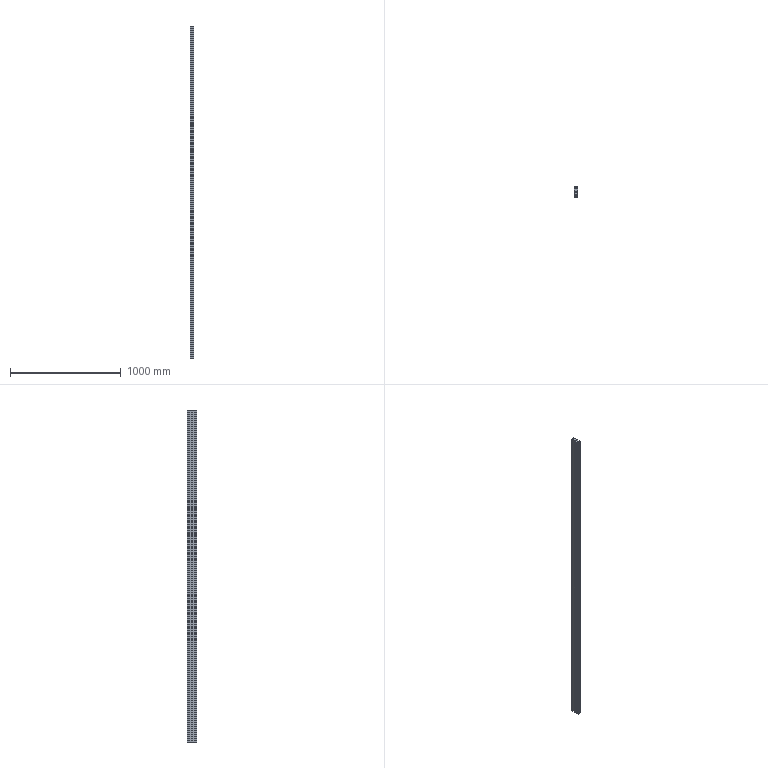Part | SolidWorks | features BaseBody 1 | 1 solid | 38 faces | box 30 x 90 x 3000 mm | volume 6756000 mm3 | plane 38
STEP:
#1=CARTESIAN_POINT('',(8.,-4.,3000.));
#2=VERTEX_POINT('',#1);
#3=CARTESIAN_POINT('',(15.,-4.,3000.));
#4=VERTEX_POINT('',#3);
#5=CARTESIAN_POINT('',(8.,-4.,3000.));
#6=DIRECTION('',(1.,0.,0.));
#7=VECTOR('',#6,1000.);
#8=LINE('',#5,#7);
#9=EDGE_CURVE('',#2,#4,#8,.T.);
#10=ORIENTED_EDGE('',*,*,#9,.T.);
#11=CARTESIAN_POINT('',(15.,-4.,0.));
#12=VERTEX_POINT('',#11);
#13=CARTESIAN_POINT('',(15.,-4.,0.));
#14=DIRECTION('',(0.,0.,1.));
#15=VECTOR('',#14,1000.);
#16=LINE('',#13,#15);
#17=EDGE_CURVE('',#12,#4,#16,.T.);
#18=ORIENTED_EDGE('',*,*,#17,.F.);
#19=CARTESIAN_POINT('',(8.,-4.,0.));
#20=VERTEX_POINT('',#19);
#21=CARTESIAN_POINT('',(8.,-4.,0.));
#22=DIRECTION('',(1.,0.,0.));
#23=VECTOR('',#22,1000.);
#24=LINE('',#21,#23);
#25=EDGE_CURVE('',#20,#12,#24,.T.);
#26=ORIENTED_EDGE('',*,*,#25,.F.);
#27=CARTESIAN_POINT('',(8.,-4.,0.));
#28=DIRECTION('',(0.,0.,1.));
#29=VECTOR('',#28,1000.);
#30=LINE('',#27,#29);
#31=EDGE_CURVE('',#20,#2,#30,.T.);
#32=ORIENTED_EDGE('',*,*,#31,.T.);
#33=EDGE_LOOP('',(#10,#18,#26,#32));
#34=FACE_OUTER_BOUND('',#33,.T.);
#35=CARTESIAN_POINT('',(8.,-4.,0.));
#36=DIRECTION('',(0.,-1.,0.));
#37=DIRECTION('',(0.,0.,-1.));
#38=AXIS2_PLACEMENT_3D('',#35,#36,#37);
#39=PLANE('',#38);
#40=ADVANCED_FACE('',(#34),#39,.F.);
#41=CARTESIAN_POINT('',(15.,4.,3000.));
#42=VERTEX_POINT('',#41);
#43=CARTESIAN_POINT('',(8.,4.,3000.));
#44=VERTEX_POINT('',#43);
#45=CARTESIAN_POINT('',(8.,4.,3000.));
#46=DIRECTION('',(-1.,0.,0.));
#47=VECTOR('',#46,1000.);
#48=LINE('',#45,#47);
#49=EDGE_CURVE('',#42,#44,#48,.T.);
#50=ORIENTED_EDGE('',*,*,#49,.T.);
#51=CARTESIAN_POINT('',(8.,4.,0.));
#52=VERTEX_POINT('',#51);
#53=CARTESIAN_POINT('',(8.,4.,0.));
#54=DIRECTION('',(0.,0.,1.));
#55=VECTOR('',#54,1000.);
#56=LINE('',#53,#55);
#57=EDGE_CURVE('',#52,#44,#56,.T.);
#58=ORIENTED_EDGE('',*,*,#57,.F.);
#59=CARTESIAN_POINT('',(15.,4.,0.));
#60=VERTEX_POINT('',#59);
#61=CARTESIAN_POINT('',(8.,4.,0.));
#62=DIRECTION('',(-1.,0.,0.));
#63=VECTOR('',#62,1000.);
#64=LINE('',#61,#63);
#65=EDGE_CURVE('',#60,#52,#64,.T.);
#66=ORIENTED_EDGE('',*,*,#65,.F.);
#67=CARTESIAN_POINT('',(15.,4.,0.));
#68=DIRECTION('',(0.,0.,1.));
#69=VECTOR('',#68,1000.);
#70=LINE('',#67,#69);
#71=EDGE_CURVE('',#60,#42,#70,.T.);
#72=ORIENTED_EDGE('',*,*,#71,.T.);
#73=EDGE_LOOP('',(#50,#58,#66,#72));
#74=FACE_OUTER_BOUND('',#73,.T.);
#75=CARTESIAN_POINT('',(8.,4.,0.));
#76=DIRECTION('',(0.,1.,0.));
#77=DIRECTION('',(1.,0.,0.));
#78=AXIS2_PLACEMENT_3D('',#75,#76,#77);
#79=PLANE('',#78);
#80=ADVANCED_FACE('',(#74),#79,.F.);
#81=CARTESIAN_POINT('',(8.,-4.,3000.));
#82=DIRECTION('',(0.,-1.,0.));
#83=VECTOR('',#82,1000.);
#84=LINE('',#81,#83);
#85=EDGE_CURVE('',#44,#2,#84,.T.);
#86=ORIENTED_EDGE('',*,*,#85,.T.);
#87=ORIENTED_EDGE('',*,*,#31,.F.);
#88=CARTESIAN_POINT('',(8.,-4.,0.));
#89=DIRECTION('',(0.,-1.,0.));
#90=VECTOR('',#89,1000.);
#91=LINE('',#88,#90);
#92=EDGE_CURVE('',#52,#20,#91,.T.);
#93=ORIENTED_EDGE('',*,*,#92,.F.);
#94=ORIENTED_EDGE('',*,*,#57,.T.);
#95=EDGE_LOOP('',(#86,#87,#93,#94));
#96=FACE_OUTER_BOUND('',#95,.T.);
#97=CARTESIAN_POINT('',(8.,-4.,0.));
#98=DIRECTION('',(-1.,0.,0.));
#99=DIRECTION('',(0.,0.,1.));
#100=AXIS2_PLACEMENT_3D('',#97,#98,#99);
#101=PLANE('',#100);
#102=ADVANCED_FACE('',(#96),#101,.F.);
#103=CARTESIAN_POINT('',(-15.,-4.,3000.));
#104=VERTEX_POINT('',#103);
#105=CARTESIAN_POINT('',(-8.,-4.,3000.));
#106=VERTEX_POINT('',#105);
#107=CARTESIAN_POINT('',(-15.,-4.,3000.));
#108=DIRECTION('',(1.,0.,0.));
#109=VECTOR('',#108,1000.);
#110=LINE('',#107,#109);
#111=EDGE_CURVE('',#104,#106,#110,.T.);
#112=ORIENTED_EDGE('',*,*,#111,.T.);
#113=CARTESIAN_POINT('',(-8.,-4.,0.));
#114=VERTEX_POINT('',#113);
#115=CARTESIAN_POINT('',(-8.,-4.,0.));
#116=DIRECTION('',(0.,0.,1.));
#117=VECTOR('',#116,1000.);
#118=LINE('',#115,#117);
#119=EDGE_CURVE('',#114,#106,#118,.T.);
#120=ORIENTED_EDGE('',*,*,#119,.F.);
#121=CARTESIAN_POINT('',(-15.,-4.,0.));
#122=VERTEX_POINT('',#121);
#123=CARTESIAN_POINT('',(-15.,-4.,0.));
#124=DIRECTION('',(1.,0.,0.));
#125=VECTOR('',#124,1000.);
#126=LINE('',#123,#125);
#127=EDGE_CURVE('',#122,#114,#126,.T.);
#128=ORIENTED_EDGE('',*,*,#127,.F.);
#129=CARTESIAN_POINT('',(-15.,-4.,0.));
#130=DIRECTION('',(0.,0.,1.));
#131=VECTOR('',#130,1000.);
#132=LINE('',#129,#131);
#133=EDGE_CURVE('',#122,#104,#132,.T.);
#134=ORIENTED_EDGE('',*,*,#133,.T.);
#135=EDGE_LOOP('',(#112,#120,#128,#134));
#136=FACE_OUTER_BOUND('',#135,.T.);
#137=CARTESIAN_POINT('',(-15.,-4.,0.));
#138=DIRECTION('',(0.,-1.,0.));
#139=DIRECTION('',(0.,0.,-1.));
#140=AXIS2_PLACEMENT_3D('',#137,#138,#139);
#141=PLANE('',#140);
#142=ADVANCED_FACE('',(#136),#141,.F.);
#143=CARTESIAN_POINT('',(-8.,4.,3000.));
#144=VERTEX_POINT('',#143);
#145=CARTESIAN_POINT('',(-8.,-4.,3000.));
#146=DIRECTION('',(0.,1.,0.));
#147=VECTOR('',#146,1000.);
#148=LINE('',#145,#147);
#149=EDGE_CURVE('',#106,#144,#148,.T.);
#150=ORIENTED_EDGE('',*,*,#149,.T.);
#151=CARTESIAN_POINT('',(-8.,4.,0.));
#152=VERTEX_POINT('',#151);
#153=CARTESIAN_POINT('',(-8.,4.,0.));
#154=DIRECTION('',(0.,0.,1.));
#155=VECTOR('',#154,1000.);
#156=LINE('',#153,#155);
#157=EDGE_CURVE('',#152,#144,#156,.T.);
#158=ORIENTED_EDGE('',*,*,#157,.F.);
#159=CARTESIAN_POINT('',(-8.,-4.,0.));
#160=DIRECTION('',(0.,1.,0.));
#161=VECTOR('',#160,1000.);
#162=LINE('',#159,#161);
#163=EDGE_CURVE('',#114,#152,#162,.T.);
#164=ORIENTED_EDGE('',*,*,#163,.F.);
#165=ORIENTED_EDGE('',*,*,#119,.T.);
#166=EDGE_LOOP('',(#150,#158,#164,#165));
#167=FACE_OUTER_BOUND('',#166,.T.);
#168=CARTESIAN_POINT('',(-8.,-4.,0.));
#169=DIRECTION('',(1.,0.,0.));
#170=DIRECTION('',(0.,1.,0.));
#171=AXIS2_PLACEMENT_3D('',#168,#169,#170);
#172=PLANE('',#171);
#173=ADVANCED_FACE('',(#167),#172,.F.);
#174=CARTESIAN_POINT('',(-15.,4.,3000.));
#175=VERTEX_POINT('',#174);
#176=CARTESIAN_POINT('',(-15.,4.,3000.));
#177=DIRECTION('',(-1.,0.,0.));
#178=VECTOR('',#177,1000.);
#179=LINE('',#176,#178);
#180=EDGE_CURVE('',#144,#175,#179,.T.);
#181=ORIENTED_EDGE('',*,*,#180,.T.);
#182=CARTESIAN_POINT('',(-15.,4.,0.));
#183=VERTEX_POINT('',#182);
#184=CARTESIAN_POINT('',(-15.,4.,0.));
#185=DIRECTION('',(0.,0.,1.));
#186=VECTOR('',#185,1000.);
#187=LINE('',#184,#186);
#188=EDGE_CURVE('',#183,#175,#187,.T.);
#189=ORIENTED_EDGE('',*,*,#188,.F.);
#190=CARTESIAN_POINT('',(-15.,4.,0.));
#191=DIRECTION('',(-1.,0.,0.));
#192=VECTOR('',#191,1000.);
#193=LINE('',#190,#192);
#194=EDGE_CURVE('',#152,#183,#193,.T.);
#195=ORIENTED_EDGE('',*,*,#194,.F.);
#196=ORIENTED_EDGE('',*,*,#157,.T.);
#197=EDGE_LOOP('',(#181,#189,#195,#196));
#198=FACE_OUTER_BOUND('',#197,.T.);
#199=CARTESIAN_POINT('',(-15.,4.,0.));
#200=DIRECTION('',(0.,1.,0.));
#201=DIRECTION('',(1.,0.,0.));
#202=AXIS2_PLACEMENT_3D('',#199,#200,#201);
#203=PLANE('',#202);
#204=ADVANCED_FACE('',(#198),#203,.F.);
#205=CARTESIAN_POINT('',(15.,-26.,3000.));
#206=VERTEX_POINT('',#205);
#207=CARTESIAN_POINT('',(8.,-26.,3000.));
#208=VERTEX_POINT('',#207);
#209=CARTESIAN_POINT('',(8.,-26.,3000.));
#210=DIRECTION('',(-1.,0.,0.));
#211=VECTOR('',#210,1000.);
#212=LINE('',#209,#211);
#213=EDGE_CURVE('',#206,#208,#212,.T.);
#214=ORIENTED_EDGE('',*,*,#213,.T.);
#215=CARTESIAN_POINT('',(8.,-26.,0.));
#216=VERTEX_POINT('',#215);
#217=CARTESIAN_POINT('',(8.,-26.,0.));
#218=DIRECTION('',(0.,0.,1.));
#219=VECTOR('',#218,1000.);
#220=LINE('',#217,#219);
#221=EDGE_CURVE('',#216,#208,#220,.T.);
#222=ORIENTED_EDGE('',*,*,#221,.F.);
#223=CARTESIAN_POINT('',(15.,-26.,0.));
#224=VERTEX_POINT('',#223);
#225=CARTESIAN_POINT('',(8.,-26.,0.));
#226=DIRECTION('',(-1.,0.,0.));
#227=VECTOR('',#226,1000.);
#228=LINE('',#225,#227);
#229=EDGE_CURVE('',#224,#216,#228,.T.);
#230=ORIENTED_EDGE('',*,*,#229,.F.);
#231=CARTESIAN_POINT('',(15.,-26.,0.));
#232=DIRECTION('',(0.,0.,1.));
#233=VECTOR('',#232,1000.);
#234=LINE('',#231,#233);
#235=EDGE_CURVE('',#224,#206,#234,.T.);
#236=ORIENTED_EDGE('',*,*,#235,.T.);
#237=EDGE_LOOP('',(#214,#222,#230,#236));
#238=FACE_OUTER_BOUND('',#237,.T.);
#239=CARTESIAN_POINT('',(8.,-26.,0.));
#240=DIRECTION('',(0.,1.,0.));
#241=DIRECTION('',(1.,0.,0.));
#242=AXIS2_PLACEMENT_3D('',#239,#240,#241);
#243=PLANE('',#242);
#244=ADVANCED_FACE('',(#238),#243,.F.);
#245=CARTESIAN_POINT('',(8.,-34.,3000.));
#246=VERTEX_POINT('',#245);
#247=CARTESIAN_POINT('',(8.,-26.,3000.));
#248=DIRECTION('',(0.,-1.,0.));
#249=VECTOR('',#248,1000.);
#250=LINE('',#247,#249);
#251=EDGE_CURVE('',#208,#246,#250,.T.);
#252=ORIENTED_EDGE('',*,*,#251,.T.);
#253=CARTESIAN_POINT('',(8.,-34.,0.));
#254=VERTEX_POINT('',#253);
#255=CARTESIAN_POINT('',(8.,-34.,0.));
#256=DIRECTION('',(0.,0.,1.));
#257=VECTOR('',#256,1000.);
#258=LINE('',#255,#257);
#259=EDGE_CURVE('',#254,#246,#258,.T.);
#260=ORIENTED_EDGE('',*,*,#259,.F.);
#261=CARTESIAN_POINT('',(8.,-26.,0.));
#262=DIRECTION('',(0.,-1.,0.));
#263=VECTOR('',#262,1000.);
#264=LINE('',#261,#263);
#265=EDGE_CURVE('',#216,#254,#264,.T.);
#266=ORIENTED_EDGE('',*,*,#265,.F.);
#267=ORIENTED_EDGE('',*,*,#221,.T.);
#268=EDGE_LOOP('',(#252,#260,#266,#267));
#269=FACE_OUTER_BOUND('',#268,.T.);
#270=CARTESIAN_POINT('',(8.,-26.,0.));
#271=DIRECTION('',(-1.,0.,0.));
#272=DIRECTION('',(0.,1.,0.));
#273=AXIS2_PLACEMENT_3D('',#270,#271,#272);
#274=PLANE('',#273);
#275=ADVANCED_FACE('',(#269),#274,.F.);
#276=CARTESIAN_POINT('',(15.,-34.,3000.));
#277=VERTEX_POINT('',#276);
#278=CARTESIAN_POINT('',(8.,-34.,3000.));
#279=DIRECTION('',(1.,0.,0.));
#280=VECTOR('',#279,1000.);
#281=LINE('',#278,#280);
#282=EDGE_CURVE('',#246,#277,#281,.T.);
#283=ORIENTED_EDGE('',*,*,#282,.T.);
#284=CARTESIAN_POINT('',(15.,-34.,0.));
#285=VERTEX_POINT('',#284);
#286=CARTESIAN_POINT('',(15.,-34.,0.));
#287=DIRECTION('',(0.,0.,1.));
#288=VECTOR('',#287,1000.);
#289=LINE('',#286,#288);
#290=EDGE_CURVE('',#285,#277,#289,.T.);
#291=ORIENTED_EDGE('',*,*,#290,.F.);
#292=CARTESIAN_POINT('',(8.,-34.,0.));
#293=DIRECTION('',(1.,0.,0.));
#294=VECTOR('',#293,1000.);
#295=LINE('',#292,#294);
#296=EDGE_CURVE('',#254,#285,#295,.T.);
#297=ORIENTED_EDGE('',*,*,#296,.F.);
#298=ORIENTED_EDGE('',*,*,#259,.T.);
#299=EDGE_LOOP('',(#283,#291,#297,#298));
#300=FACE_OUTER_BOUND('',#299,.T.);
#301=CARTESIAN_POINT('',(8.,-34.,0.));
#302=DIRECTION('',(0.,-1.,0.));
#303=DIRECTION('',(0.,0.,-1.));
#304=AXIS2_PLACEMENT_3D('',#301,#302,#303);
#305=PLANE('',#304);
#306=ADVANCED_FACE('',(#300),#305,.F.);
#307=CARTESIAN_POINT('',(-15.,-34.,3000.));
#308=VERTEX_POINT('',#307);
#309=CARTESIAN_POINT('',(-8.,-34.,3000.));
#310=VERTEX_POINT('',#309);
#311=CARTESIAN_POINT('',(-15.,-34.,3000.));
#312=DIRECTION('',(1.,0.,0.));
#313=VECTOR('',#312,1000.);
#314=LINE('',#311,#313);
#315=EDGE_CURVE('',#308,#310,#314,.T.);
#316=ORIENTED_EDGE('',*,*,#315,.T.);
#317=CARTESIAN_POINT('',(-8.,-34.,0.));
#318=VERTEX_POINT('',#317);
#319=CARTESIAN_POINT('',(-8.,-34.,0.));
#320=DIRECTION('',(0.,0.,1.));
#321=VECTOR('',#320,1000.);
#322=LINE('',#319,#321);
#323=EDGE_CURVE('',#318,#310,#322,.T.);
#324=ORIENTED_EDGE('',*,*,#323,.F.);
#325=CARTESIAN_POINT('',(-15.,-34.,0.));
#326=VERTEX_POINT('',#325);
#327=CARTESIAN_POINT('',(-15.,-34.,0.));
#328=DIRECTION('',(1.,0.,0.));
#329=VECTOR('',#328,1000.);
#330=LINE('',#327,#329);
#331=EDGE_CURVE('',#326,#318,#330,.T.);
#332=ORIENTED_EDGE('',*,*,#331,.F.);
#333=CARTESIAN_POINT('',(-15.,-34.,0.));
#334=DIRECTION('',(0.,0.,1.));
#335=VECTOR('',#334,1000.);
#336=LINE('',#333,#335);
#337=EDGE_CURVE('',#326,#308,#336,.T.);
#338=ORIENTED_EDGE('',*,*,#337,.T.);
#339=EDGE_LOOP('',(#316,#324,#332,#338));
#340=FACE_OUTER_BOUND('',#339,.T.);
#341=CARTESIAN_POINT('',(-15.,-34.,0.));
#342=DIRECTION('',(0.,-1.,0.));
#343=DIRECTION('',(0.,0.,-1.));
#344=AXIS2_PLACEMENT_3D('',#341,#342,#343);
#345=PLANE('',#344);
#346=ADVANCED_FACE('',(#340),#345,.F.);
#347=CARTESIAN_POINT('',(-8.,-26.,3000.));
#348=VERTEX_POINT('',#347);
#349=CARTESIAN_POINT('',(-8.,-26.,3000.));
#350=DIRECTION('',(0.,1.,0.));
#351=VECTOR('',#350,1000.);
#352=LINE('',#349,#351);
#353=EDGE_CURVE('',#310,#348,#352,.T.);
#354=ORIENTED_EDGE('',*,*,#353,.T.);
#355=CARTESIAN_POINT('',(-8.,-26.,0.));
#356=VERTEX_POINT('',#355);
#357=CARTESIAN_POINT('',(-8.,-26.,0.));
#358=DIRECTION('',(0.,0.,1.));
#359=VECTOR('',#358,1000.);
#360=LINE('',#357,#359);
#361=EDGE_CURVE('',#356,#348,#360,.T.);
#362=ORIENTED_EDGE('',*,*,#361,.F.);
#363=CARTESIAN_POINT('',(-8.,-26.,0.));
#364=DIRECTION('',(0.,1.,0.));
#365=VECTOR('',#364,1000.);
#366=LINE('',#363,#365);
#367=EDGE_CURVE('',#318,#356,#366,.T.);
#368=ORIENTED_EDGE('',*,*,#367,.F.);
#369=ORIENTED_EDGE('',*,*,#323,.T.);
#370=EDGE_LOOP('',(#354,#362,#368,#369));
#371=FACE_OUTER_BOUND('',#370,.T.);
#372=CARTESIAN_POINT('',(-8.,-26.,0.));
#373=DIRECTION('',(1.,0.,0.));
#374=DIRECTION('',(0.,1.,0.));
#375=AXIS2_PLACEMENT_3D('',#372,#373,#374);
#376=PLANE('',#375);
#377=ADVANCED_FACE('',(#371),#376,.F.);
#378=CARTESIAN_POINT('',(-15.,-26.,3000.));
#379=VERTEX_POINT('',#378);
#380=CARTESIAN_POINT('',(-15.,-26.,3000.));
#381=DIRECTION('',(-1.,0.,0.));
#382=VECTOR('',#381,1000.);
#383=LINE('',#380,#382);
#384=EDGE_CURVE('',#348,#379,#383,.T.);
#385=ORIENTED_EDGE('',*,*,#384,.T.);
#386=CARTESIAN_POINT('',(-15.,-26.,0.));
#387=VERTEX_POINT('',#386);
#388=CARTESIAN_POINT('',(-15.,-26.,0.));
#389=DIRECTION('',(0.,0.,1.));
#390=VECTOR('',#389,1000.);
#391=LINE('',#388,#390);
#392=EDGE_CURVE('',#387,#379,#391,.T.);
#393=ORIENTED_EDGE('',*,*,#392,.F.);
#394=CARTESIAN_POINT('',(-15.,-26.,0.));
#395=DIRECTION('',(-1.,0.,0.));
#396=VECTOR('',#395,1000.);
#397=LINE('',#394,#396);
#398=EDGE_CURVE('',#356,#387,#397,.T.);
#399=ORIENTED_EDGE('',*,*,#398,.F.);
#400=ORIENTED_EDGE('',*,*,#361,.T.);
#401=EDGE_LOOP('',(#385,#393,#399,#400));
#402=FACE_OUTER_BOUND('',#401,.T.);
#403=CARTESIAN_POINT('',(-15.,-26.,0.));
#404=DIRECTION('',(0.,1.,0.));
#405=DIRECTION('',(1.,0.,0.));
#406=AXIS2_PLACEMENT_3D('',#403,#404,#405);
#407=PLANE('',#406);
#408=ADVANCED_FACE('',(#402),#407,.F.);
#409=CARTESIAN_POINT('',(15.,34.,3000.));
#410=VERTEX_POINT('',#409);
#411=CARTESIAN_POINT('',(8.,34.,3000.));
#412=VERTEX_POINT('',#411);
#413=CARTESIAN_POINT('',(8.,34.,3000.));
#414=DIRECTION('',(-1.,0.,0.));
#415=VECTOR('',#414,1000.);
#416=LINE('',#413,#415);
#417=EDGE_CURVE('',#410,#412,#416,.T.);
#418=ORIENTED_EDGE('',*,*,#417,.T.);
#419=CARTESIAN_POINT('',(8.,34.,0.));
#420=VERTEX_POINT('',#419);
#421=CARTESIAN_POINT('',(8.,34.,0.));
#422=DIRECTION('',(0.,0.,1.));
#423=VECTOR('',#422,1000.);
#424=LINE('',#421,#423);
#425=EDGE_CURVE('',#420,#412,#424,.T.);
#426=ORIENTED_EDGE('',*,*,#425,.F.);
#427=CARTESIAN_POINT('',(15.,34.,0.));
#428=VERTEX_POINT('',#427);
#429=CARTESIAN_POINT('',(8.,34.,0.));
#430=DIRECTION('',(-1.,0.,0.));
#431=VECTOR('',#430,1000.);
#432=LINE('',#429,#431);
#433=EDGE_CURVE('',#428,#420,#432,.T.);
#434=ORIENTED_EDGE('',*,*,#433,.F.);
#435=CARTESIAN_POINT('',(15.,34.,0.));
#436=DIRECTION('',(0.,0.,1.));
#437=VECTOR('',#436,1000.);
#438=LINE('',#435,#437);
#439=EDGE_CURVE('',#428,#410,#438,.T.);
#440=ORIENTED_EDGE('',*,*,#439,.T.);
#441=EDGE_LOOP('',(#418,#426,#434,#440));
#442=FACE_OUTER_BOUND('',#441,.T.);
#443=CARTESIAN_POINT('',(8.,34.,0.));
#444=DIRECTION('',(0.,1.,0.));
#445=DIRECTION('',(1.,0.,0.));
#446=AXIS2_PLACEMENT_3D('',#443,#444,#445);
#447=PLANE('',#446);
#448=ADVANCED_FACE('',(#442),#447,.F.);
#449=CARTESIAN_POINT('',(8.,26.,3000.));
#450=VERTEX_POINT('',#449);
#451=CARTESIAN_POINT('',(8.,34.,3000.));
#452=DIRECTION('',(0.,-1.,0.));
#453=VECTOR('',#452,1000.);
#454=LINE('',#451,#453);
#455=EDGE_CURVE('',#412,#450,#454,.T.);
#456=ORIENTED_EDGE('',*,*,#455,.T.);
#457=CARTESIAN_POINT('',(8.,26.,0.));
#458=VERTEX_POINT('',#457);
#459=CARTESIAN_POINT('',(8.,26.,0.));
#460=DIRECTION('',(0.,0.,1.));
#461=VECTOR('',#460,1000.);
#462=LINE('',#459,#461);
#463=EDGE_CURVE('',#458,#450,#462,.T.);
#464=ORIENTED_EDGE('',*,*,#463,.F.);
#465=CARTESIAN_POINT('',(8.,34.,0.));
#466=DIRECTION('',(0.,-1.,0.));
#467=VECTOR('',#466,1000.);
#468=LINE('',#465,#467);
#469=EDGE_CURVE('',#420,#458,#468,.T.);
#470=ORIENTED_EDGE('',*,*,#469,.F.);
#471=ORIENTED_EDGE('',*,*,#425,.T.);
#472=EDGE_LOOP('',(#456,#464,#470,#471));
#473=FACE_OUTER_BOUND('',#472,.T.);
#474=CARTESIAN_POINT('',(8.,34.,0.));
#475=DIRECTION('',(-1.,0.,0.));
#476=DIRECTION('',(0.,1.,0.));
#477=AXIS2_PLACEMENT_3D('',#474,#475,#476);
#478=PLANE('',#477);
#479=ADVANCED_FACE('',(#473),#478,.F.);
#480=CARTESIAN_POINT('',(15.,26.,3000.));
#481=VERTEX_POINT('',#480);
#482=CARTESIAN_POINT('',(8.,26.,3000.));
#483=DIRECTION('',(1.,0.,0.));
#484=VECTOR('',#483,1000.);
#485=LINE('',#482,#484);
#486=EDGE_CURVE('',#450,#481,#485,.T.);
#487=ORIENTED_EDGE('',*,*,#486,.T.);
#488=CARTESIAN_POINT('',(15.,26.,0.));
#489=VERTEX_POINT('',#488);
#490=CARTESIAN_POINT('',(15.,26.,0.));
#491=DIRECTION('',(0.,0.,1.));
#492=VECTOR('',#491,1000.);
#493=LINE('',#490,#492);
#494=EDGE_CURVE('',#489,#481,#493,.T.);
#495=ORIENTED_EDGE('',*,*,#494,.F.);
#496=CARTESIAN_POINT('',(8.,26.,0.));
#497=DIRECTION('',(1.,0.,0.));
#498=VECTOR('',#497,1000.);
#499=LINE('',#496,#498);
#500=EDGE_CURVE('',#458,#489,#499,.T.);
#501=ORIENTED_EDGE('',*,*,#500,.F.);
#502=ORIENTED_EDGE('',*,*,#463,.T.);
#503=EDGE_LOOP('',(#487,#495,#501,#502));
#504=FACE_OUTER_BOUND('',#503,.T.);
#505=CARTESIAN_POINT('',(8.,26.,0.));
#506=DIRECTION('',(0.,-1.,0.));
#507=DIRECTION('',(0.,0.,-1.));
#508=AXIS2_PLACEMENT_3D('',#505,#506,#507);
#509=PLANE('',#508);
#510=ADVANCED_FACE('',(#504),#509,.F.);
#511=CARTESIAN_POINT('',(-15.,26.,3000.));
#512=VERTEX_POINT('',#511);
#513=CARTESIAN_POINT('',(-8.,26.,3000.));
#514=VERTEX_POINT('',#513);
#515=CARTESIAN_POINT('',(-15.,26.,3000.));
#516=DIRECTION('',(1.,0.,0.));
#517=VECTOR('',#516,1000.);
#518=LINE('',#515,#517);
#519=EDGE_CURVE('',#512,#514,#518,.T.);
#520=ORIENTED_EDGE('',*,*,#519,.T.);
#521=CARTESIAN_POINT('',(-8.,26.,0.));
#522=VERTEX_POINT('',#521);
#523=CARTESIAN_POINT('',(-8.,26.,0.));
#524=DIRECTION('',(0.,0.,1.));
#525=VECTOR('',#524,1000.);
#526=LINE('',#523,#525);
#527=EDGE_CURVE('',#522,#514,#526,.T.);
#528=ORIENTED_EDGE('',*,*,#527,.F.);
#529=CARTESIAN_POINT('',(-15.,26.,0.));
#530=VERTEX_POINT('',#529);
#531=CARTESIAN_POINT('',(-15.,26.,0.));
#532=DIRECTION('',(1.,0.,0.));
#533=VECTOR('',#532,1000.);
#534=LINE('',#531,#533);
#535=EDGE_CURVE('',#530,#522,#534,.T.);
#536=ORIENTED_EDGE('',*,*,#535,.F.);
#537=CARTESIAN_POINT('',(-15.,26.,0.));
#538=DIRECTION('',(0.,0.,1.));
#539=VECTOR('',#538,1000.);
#540=LINE('',#537,#539);
#541=EDGE_CURVE('',#530,#512,#540,.T.);
#542=ORIENTED_EDGE('',*,*,#541,.T.);
#543=EDGE_LOOP('',(#520,#528,#536,#542));
#544=FACE_OUTER_BOUND('',#543,.T.);
#545=CARTESIAN_POINT('',(-15.,26.,0.));
#546=DIRECTION('',(0.,-1.,0.));
#547=DIRECTION('',(0.,0.,-1.));
#548=AXIS2_PLACEMENT_3D('',#545,#546,#547);
#549=PLANE('',#548);
#550=ADVANCED_FACE('',(#544),#549,.F.);
#551=CARTESIAN_POINT('',(-8.,34.,3000.));
#552=VERTEX_POINT('',#551);
#553=CARTESIAN_POINT('',(-8.,34.,3000.));
#554=DIRECTION('',(0.,1.,0.));
#555=VECTOR('',#554,1000.);
#556=LINE('',#553,#555);
#557=EDGE_CURVE('',#514,#552,#556,.T.);
#558=ORIENTED_EDGE('',*,*,#557,.T.);
#559=CARTESIAN_POINT('',(-8.,34.,0.));
#560=VERTEX_POINT('',#559);
#561=CARTESIAN_POINT('',(-8.,34.,0.));
#562=DIRECTION('',(0.,0.,1.));
#563=VECTOR('',#562,1000.);
#564=LINE('',#561,#563);
#565=EDGE_CURVE('',#560,#552,#564,.T.);
#566=ORIENTED_EDGE('',*,*,#565,.F.);
#567=CARTESIAN_POINT('',(-8.,34.,0.));
#568=DIRECTION('',(0.,1.,0.));
#569=VECTOR('',#568,1000.);
#570=LINE('',#567,#569);
#571=EDGE_CURVE('',#522,#560,#570,.T.);
#572=ORIENTED_EDGE('',*,*,#571,.F.);
#573=ORIENTED_EDGE('',*,*,#527,.T.);
#574=EDGE_LOOP('',(#558,#566,#572,#573));
#575=FACE_OUTER_BOUND('',#574,.T.);
#576=CARTESIAN_POINT('',(-8.,34.,0.));
#577=DIRECTION('',(1.,0.,0.));
#578=DIRECTION('',(0.,1.,0.));
#579=AXIS2_PLACEMENT_3D('',#576,#577,#578);
#580=PLANE('',#579);
#581=ADVANCED_FACE('',(#575),#580,.F.);
#582=CARTESIAN_POINT('',(-15.,34.,3000.));
#583=VERTEX_POINT('',#582);
#584=CARTESIAN_POINT('',(-15.,34.,3000.));
#585=DIRECTION('',(-1.,0.,0.));
#586=VECTOR('',#585,1000.);
#587=LINE('',#584,#586);
#588=EDGE_CURVE('',#552,#583,#587,.T.);
#589=ORIENTED_EDGE('',*,*,#588,.T.);
#590=CARTESIAN_POINT('',(-15.,34.,0.));
#591=VERTEX_POINT('',#590);
#592=CARTESIAN_POINT('',(-15.,34.,0.));
#593=DIRECTION('',(0.,0.,1.));
#594=VECTOR('',#593,1000.);
#595=LINE('',#592,#594);
#596=EDGE_CURVE('',#591,#583,#595,.T.);
#597=ORIENTED_EDGE('',*,*,#596,.F.);
#598=CARTESIAN_POINT('',(-15.,34.,0.));
#599=DIRECTION('',(-1.,0.,0.));
#600=VECTOR('',#599,1000.);
#601=LINE('',#598,#600);
#602=EDGE_CURVE('',#560,#591,#601,.T.);
#603=ORIENTED_EDGE('',*,*,#602,.F.);
#604=ORIENTED_EDGE('',*,*,#565,.T.);
#605=EDGE_LOOP('',(#589,#597,#603,#604));
#606=FACE_OUTER_BOUND('',#605,.T.);
#607=CARTESIAN_POINT('',(-15.,34.,0.));
#608=DIRECTION('',(0.,1.,0.));
#609=DIRECTION('',(1.,0.,0.));
#610=AXIS2_PLACEMENT_3D('',#607,#608,#609);
#611=PLANE('',#610);
#612=ADVANCED_FACE('',(#606),#611,.F.);
#613=CARTESIAN_POINT('',(4.,-45.,3000.));
#614=VERTEX_POINT('',#613);
#615=CARTESIAN_POINT('',(4.,-38.,3000.));
#616=VERTEX_POINT('',#615);
#617=CARTESIAN_POINT('',(4.,-38.,3000.));
#618=DIRECTION('',(0.,1.,0.));
#619=VECTOR('',#618,1000.);
#620=LINE('',#617,#619);
#621=EDGE_CURVE('',#614,#616,#620,.T.);
#622=ORIENTED_EDGE('',*,*,#621,.T.);
#623=CARTESIAN_POINT('',(4.,-38.,0.));
#624=VERTEX_POINT('',#623);
#625=CARTESIAN_POINT('',(4.,-38.,0.));
#626=DIRECTION('',(0.,0.,1.));
#627=VECTOR('',#626,1000.);
#628=LINE('',#625,#627);
#629=EDGE_CURVE('',#624,#616,#628,.T.);
#630=ORIENTED_EDGE('',*,*,#629,.F.);
#631=CARTESIAN_POINT('',(4.,-45.,0.));
#632=VERTEX_POINT('',#631);
#633=CARTESIAN_POINT('',(4.,-38.,0.));
#634=DIRECTION('',(0.,1.,0.));
#635=VECTOR('',#634,1000.);
#636=LINE('',#633,#635);
#637=EDGE_CURVE('',#632,#624,#636,.T.);
#638=ORIENTED_EDGE('',*,*,#637,.F.);
#639=CARTESIAN_POINT('',(4.,-45.,0.));
#640=DIRECTION('',(0.,0.,1.));
#641=VECTOR('',#640,1000.);
#642=LINE('',#639,#641);
#643=EDGE_CURVE('',#632,#614,#642,.T.);
#644=ORIENTED_EDGE('',*,*,#643,.T.);
#645=EDGE_LOOP('',(#622,#630,#638,#644));
#646=FACE_OUTER_BOUND('',#645,.T.);
#647=CARTESIAN_POINT('',(4.,-38.,0.));
#648=DIRECTION('',(1.,0.,0.));
#649=DIRECTION('',(0.,1.,0.));
#650=AXIS2_PLACEMENT_3D('',#647,#648,#649);
#651=PLANE('',#650);
#652=ADVANCED_FACE('',(#646),#651,.F.);
#653=CARTESIAN_POINT('',(-4.,-38.,3000.));
#654=VERTEX_POINT('',#653);
#655=CARTESIAN_POINT('',(-4.,-38.,3000.));
#656=DIRECTION('',(-1.,0.,0.));
#657=VECTOR('',#656,1000.);
#658=LINE('',#655,#657);
#659=EDGE_CURVE('',#616,#654,#658,.T.);
#660=ORIENTED_EDGE('',*,*,#659,.T.);
#661=CARTESIAN_POINT('',(-4.,-38.,0.));
#662=VERTEX_POINT('',#661);
#663=CARTESIAN_POINT('',(-4.,-38.,0.));
#664=DIRECTION('',(0.,0.,1.));
#665=VECTOR('',#664,1000.);
#666=LINE('',#663,#665);
#667=EDGE_CURVE('',#662,#654,#666,.T.);
#668=ORIENTED_EDGE('',*,*,#667,.F.);
#669=CARTESIAN_POINT('',(-4.,-38.,0.));
#670=DIRECTION('',(-1.,0.,0.));
#671=VECTOR('',#670,1000.);
#672=LINE('',#669,#671);
#673=EDGE_CURVE('',#624,#662,#672,.T.);
#674=ORIENTED_EDGE('',*,*,#673,.F.);
#675=ORIENTED_EDGE('',*,*,#629,.T.);
#676=EDGE_LOOP('',(#660,#668,#674,#675));
#677=FACE_OUTER_BOUND('',#676,.T.);
#678=CARTESIAN_POINT('',(-4.,-38.,0.));
#679=DIRECTION('',(0.,1.,0.));
#680=DIRECTION('',(1.,0.,0.));
#681=AXIS2_PLACEMENT_3D('',#678,#679,#680);
#682=PLANE('',#681);
#683=ADVANCED_FACE('',(#677),#682,.F.);
#684=CARTESIAN_POINT('',(-4.,-45.,3000.));
#685=VERTEX_POINT('',#684);
#686=CARTESIAN_POINT('',(-4.,-38.,3000.));
#687=DIRECTION('',(0.,-1.,0.));
#688=VECTOR('',#687,1000.);
#689=LINE('',#686,#688);
#690=EDGE_CURVE('',#654,#685,#689,.T.);
#691=ORIENTED_EDGE('',*,*,#690,.T.);
#692=CARTESIAN_POINT('',(-4.,-45.,0.));
#693=VERTEX_POINT('',#692);
#694=CARTESIAN_POINT('',(-4.,-45.,0.));
#695=DIRECTION('',(0.,0.,1.));
#696=VECTOR('',#695,1000.);
#697=LINE('',#694,#696);
#698=EDGE_CURVE('',#693,#685,#697,.T.);
#699=ORIENTED_EDGE('',*,*,#698,.F.);
#700=CARTESIAN_POINT('',(-4.,-38.,0.));
#701=DIRECTION('',(0.,-1.,0.));
#702=VECTOR('',#701,1000.);
#703=LINE('',#700,#702);
#704=EDGE_CURVE('',#662,#693,#703,.T.);
#705=ORIENTED_EDGE('',*,*,#704,.F.);
#706=ORIENTED_EDGE('',*,*,#667,.T.);
#707=EDGE_LOOP('',(#691,#699,#705,#706));
#708=FACE_OUTER_BOUND('',#707,.T.);
#709=CARTESIAN_POINT('',(-4.,-38.,0.));
#710=DIRECTION('',(-1.,0.,0.));
#711=DIRECTION('',(0.,1.,0.));
#712=AXIS2_PLACEMENT_3D('',#709,#710,#711);
#713=PLANE('',#712);
#714=ADVANCED_FACE('',(#708),#713,.F.);
#715=CARTESIAN_POINT('',(-4.,45.,3000.));
#716=VERTEX_POINT('',#715);
#717=CARTESIAN_POINT('',(-4.,38.,3000.));
#718=VERTEX_POINT('',#717);
#719=CARTESIAN_POINT('',(-4.,45.,3000.));
#720=DIRECTION('',(0.,-1.,0.));
#721=VECTOR('',#720,1000.);
#722=LINE('',#719,#721);
#723=EDGE_CURVE('',#716,#718,#722,.T.);
#724=ORIENTED_EDGE('',*,*,#723,.T.);
#725=CARTESIAN_POINT('',(-4.,38.,0.));
#726=VERTEX_POINT('',#725);
#727=CARTESIAN_POINT('',(-4.,38.,0.));
#728=DIRECTION('',(0.,0.,1.));
#729=VECTOR('',#728,1000.);
#730=LINE('',#727,#729);
#731=EDGE_CURVE('',#726,#718,#730,.T.);
#732=ORIENTED_EDGE('',*,*,#731,.F.);
#733=CARTESIAN_POINT('',(-4.,45.,0.));
#734=VERTEX_POINT('',#733);
#735=CARTESIAN_POINT('',(-4.,45.,0.));
#736=DIRECTION('',(0.,-1.,0.));
#737=VECTOR('',#736,1000.);
#738=LINE('',#735,#737);
#739=EDGE_CURVE('',#734,#726,#738,.T.);
#740=ORIENTED_EDGE('',*,*,#739,.F.);
#741=CARTESIAN_POINT('',(-4.,45.,0.));
#742=DIRECTION('',(0.,0.,1.));
#743=VECTOR('',#742,1000.);
#744=LINE('',#741,#743);
#745=EDGE_CURVE('',#734,#716,#744,.T.);
#746=ORIENTED_EDGE('',*,*,#745,.T.);
#747=EDGE_LOOP('',(#724,#732,#740,#746));
#748=FACE_OUTER_BOUND('',#747,.T.);
#749=CARTESIAN_POINT('',(-4.,45.,0.));
#750=DIRECTION('',(-1.,0.,0.));
#751=DIRECTION('',(0.,1.,0.));
#752=AXIS2_PLACEMENT_3D('',#749,#750,#751);
#753=PLANE('',#752);
#754=ADVANCED_FACE('',(#748),#753,.F.);
#755=CARTESIAN_POINT('',(4.,38.,3000.));
#756=VERTEX_POINT('',#755);
#757=CARTESIAN_POINT('',(-4.,38.,3000.));
#758=DIRECTION('',(1.,0.,0.));
#759=VECTOR('',#758,1000.);
#760=LINE('',#757,#759);
#761=EDGE_CURVE('',#718,#756,#760,.T.);
#762=ORIENTED_EDGE('',*,*,#761,.T.);
#763=CARTESIAN_POINT('',(4.,38.,0.));
#764=VERTEX_POINT('',#763);
#765=CARTESIAN_POINT('',(4.,38.,0.));
#766=DIRECTION('',(0.,0.,1.));
#767=VECTOR('',#766,1000.);
#768=LINE('',#765,#767);
#769=EDGE_CURVE('',#764,#756,#768,.T.);
#770=ORIENTED_EDGE('',*,*,#769,.F.);
#771=CARTESIAN_POINT('',(-4.,38.,0.));
#772=DIRECTION('',(1.,0.,0.));
#773=VECTOR('',#772,1000.);
#774=LINE('',#771,#773);
#775=EDGE_CURVE('',#726,#764,#774,.T.);
#776=ORIENTED_EDGE('',*,*,#775,.F.);
#777=ORIENTED_EDGE('',*,*,#731,.T.);
#778=EDGE_LOOP('',(#762,#770,#776,#777));
#779=FACE_OUTER_BOUND('',#778,.T.);
#780=CARTESIAN_POINT('',(-4.,38.,0.));
#781=DIRECTION('',(0.,-1.,0.));
#782=DIRECTION('',(0.,0.,-1.));
#783=AXIS2_PLACEMENT_3D('',#780,#781,#782);
#784=PLANE('',#783);
#785=ADVANCED_FACE('',(#779),#784,.F.);
#786=CARTESIAN_POINT('',(4.,45.,3000.));
#787=VERTEX_POINT('',#786);
#788=CARTESIAN_POINT('',(4.,45.,3000.));
#789=DIRECTION('',(0.,1.,0.));
#790=VECTOR('',#789,1000.);
#791=LINE('',#788,#790);
#792=EDGE_CURVE('',#756,#787,#791,.T.);
#793=ORIENTED_EDGE('',*,*,#792,.T.);
#794=CARTESIAN_POINT('',(4.,45.,0.));
#795=VERTEX_POINT('',#794);
#796=CARTESIAN_POINT('',(4.,45.,0.));
#797=DIRECTION('',(0.,0.,1.));
#798=VECTOR('',#797,1000.);
#799=LINE('',#796,#798);
#800=EDGE_CURVE('',#795,#787,#799,.T.);
#801=ORIENTED_EDGE('',*,*,#800,.F.);
#802=CARTESIAN_POINT('',(4.,45.,0.));
#803=DIRECTION('',(0.,1.,0.));
#804=VECTOR('',#803,1000.);
#805=LINE('',#802,#804);
#806=EDGE_CURVE('',#764,#795,#805,.T.);
#807=ORIENTED_EDGE('',*,*,#806,.F.);
#808=ORIENTED_EDGE('',*,*,#769,.T.);
#809=EDGE_LOOP('',(#793,#801,#807,#808));
#810=FACE_OUTER_BOUND('',#809,.T.);
#811=CARTESIAN_POINT('',(4.,45.,0.));
#812=DIRECTION('',(1.,0.,0.));
#813=DIRECTION('',(0.,1.,0.));
#814=AXIS2_PLACEMENT_3D('',#811,#812,#813);
#815=PLANE('',#814);
#816=ADVANCED_FACE('',(#810),#815,.F.);
#817=CARTESIAN_POINT('',(15.,45.,0.));
#818=DIRECTION('',(0.,1.,0.));
#819=VECTOR('',#818,1000.);
#820=LINE('',#817,#819);
#821=EDGE_CURVE('',#60,#489,#820,.T.);
#822=ORIENTED_EDGE('',*,*,#821,.F.);
#823=ORIENTED_EDGE('',*,*,#65,.T.);
#824=ORIENTED_EDGE('',*,*,#92,.T.);
#825=ORIENTED_EDGE('',*,*,#25,.T.);
#826=CARTESIAN_POINT('',(15.,45.,0.));
#827=DIRECTION('',(0.,1.,0.));
#828=VECTOR('',#827,1000.);
#829=LINE('',#826,#828);
#830=EDGE_CURVE('',#224,#12,#829,.T.);
#831=ORIENTED_EDGE('',*,*,#830,.F.);
#832=ORIENTED_EDGE('',*,*,#229,.T.);
#833=ORIENTED_EDGE('',*,*,#265,.T.);
#834=ORIENTED_EDGE('',*,*,#296,.T.);
#835=CARTESIAN_POINT('',(15.,-45.,0.));
#836=VERTEX_POINT('',#835);
#837=CARTESIAN_POINT('',(15.,45.,0.));
#838=DIRECTION('',(0.,1.,0.));
#839=VECTOR('',#838,1000.);
#840=LINE('',#837,#839);
#841=EDGE_CURVE('',#836,#285,#840,.T.);
#842=ORIENTED_EDGE('',*,*,#841,.F.);
#843=CARTESIAN_POINT('',(-15.,-45.,0.));
#844=DIRECTION('',(1.,0.,0.));
#845=VECTOR('',#844,1000.);
#846=LINE('',#843,#845);
#847=EDGE_CURVE('',#632,#836,#846,.T.);
#848=ORIENTED_EDGE('',*,*,#847,.F.);
#849=ORIENTED_EDGE('',*,*,#637,.T.);
#850=ORIENTED_EDGE('',*,*,#673,.T.);
#851=ORIENTED_EDGE('',*,*,#704,.T.);
#852=CARTESIAN_POINT('',(-15.,-45.,0.));
#853=VERTEX_POINT('',#852);
#854=CARTESIAN_POINT('',(-15.,-45.,0.));
#855=DIRECTION('',(1.,0.,0.));
#856=VECTOR('',#855,1000.);
#857=LINE('',#854,#856);
#858=EDGE_CURVE('',#853,#693,#857,.T.);
#859=ORIENTED_EDGE('',*,*,#858,.F.);
#860=CARTESIAN_POINT('',(-15.,45.,0.));
#861=DIRECTION('',(0.,-1.,0.));
#862=VECTOR('',#861,1000.);
#863=LINE('',#860,#862);
#864=EDGE_CURVE('',#326,#853,#863,.T.);
#865=ORIENTED_EDGE('',*,*,#864,.F.);
#866=ORIENTED_EDGE('',*,*,#331,.T.);
#867=ORIENTED_EDGE('',*,*,#367,.T.);
#868=ORIENTED_EDGE('',*,*,#398,.T.);
#869=CARTESIAN_POINT('',(-15.,45.,0.));
#870=DIRECTION('',(0.,-1.,0.));
#871=VECTOR('',#870,1000.);
#872=LINE('',#869,#871);
#873=EDGE_CURVE('',#122,#387,#872,.T.);
#874=ORIENTED_EDGE('',*,*,#873,.F.);
#875=ORIENTED_EDGE('',*,*,#127,.T.);
#876=ORIENTED_EDGE('',*,*,#163,.T.);
#877=ORIENTED_EDGE('',*,*,#194,.T.);
#878=CARTESIAN_POINT('',(-15.,45.,0.));
#879=DIRECTION('',(0.,-1.,0.));
#880=VECTOR('',#879,1000.);
#881=LINE('',#878,#880);
#882=EDGE_CURVE('',#530,#183,#881,.T.);
#883=ORIENTED_EDGE('',*,*,#882,.F.);
#884=ORIENTED_EDGE('',*,*,#535,.T.);
#885=ORIENTED_EDGE('',*,*,#571,.T.);
#886=ORIENTED_EDGE('',*,*,#602,.T.);
#887=CARTESIAN_POINT('',(-15.,45.,0.));
#888=VERTEX_POINT('',#887);
#889=CARTESIAN_POINT('',(-15.,45.,0.));
#890=DIRECTION('',(0.,-1.,0.));
#891=VECTOR('',#890,1000.);
#892=LINE('',#889,#891);
#893=EDGE_CURVE('',#888,#591,#892,.T.);
#894=ORIENTED_EDGE('',*,*,#893,.F.);
#895=CARTESIAN_POINT('',(-15.,45.,0.));
#896=DIRECTION('',(-1.,0.,0.));
#897=VECTOR('',#896,1000.);
#898=LINE('',#895,#897);
#899=EDGE_CURVE('',#734,#888,#898,.T.);
#900=ORIENTED_EDGE('',*,*,#899,.F.);
#901=ORIENTED_EDGE('',*,*,#739,.T.);
#902=ORIENTED_EDGE('',*,*,#775,.T.);
#903=ORIENTED_EDGE('',*,*,#806,.T.);
#904=CARTESIAN_POINT('',(15.,45.,0.));
#905=VERTEX_POINT('',#904);
#906=CARTESIAN_POINT('',(-15.,45.,0.));
#907=DIRECTION('',(-1.,0.,0.));
#908=VECTOR('',#907,1000.);
#909=LINE('',#906,#908);
#910=EDGE_CURVE('',#905,#795,#909,.T.);
#911=ORIENTED_EDGE('',*,*,#910,.F.);
#912=CARTESIAN_POINT('',(15.,45.,0.));
#913=DIRECTION('',(0.,1.,0.));
#914=VECTOR('',#913,1000.);
#915=LINE('',#912,#914);
#916=EDGE_CURVE('',#428,#905,#915,.T.);
#917=ORIENTED_EDGE('',*,*,#916,.F.);
#918=ORIENTED_EDGE('',*,*,#433,.T.);
#919=ORIENTED_EDGE('',*,*,#469,.T.);
#920=ORIENTED_EDGE('',*,*,#500,.T.);
#921=EDGE_LOOP('',(#822,#823,#824,#825,#831,#832,#833,#834,#842,#848,#849,#850,#851,#859,#865,#866,#867,#868,#874,#875,#876,#877,#883,#884,#885,#886,#894,#900,#901,#902,#903,#911,#917,#918,#919,#920));
#922=FACE_OUTER_BOUND('',#921,.T.);
#923=CARTESIAN_POINT('',(0.,0.,0.));
#924=DIRECTION('',(0.,0.,1.));
#925=DIRECTION('',(1.,0.,0.));
#926=AXIS2_PLACEMENT_3D('',#923,#924,#925);
#927=PLANE('',#926);
#928=ADVANCED_FACE('',(#922),#927,.F.);
#929=ORIENTED_EDGE('',*,*,#49,.F.);
#930=CARTESIAN_POINT('',(15.,45.,3000.));
#931=DIRECTION('',(0.,1.,0.));
#932=VECTOR('',#931,1000.);
#933=LINE('',#930,#932);
#934=EDGE_CURVE('',#42,#481,#933,.T.);
#935=ORIENTED_EDGE('',*,*,#934,.T.);
#936=ORIENTED_EDGE('',*,*,#486,.F.);
#937=ORIENTED_EDGE('',*,*,#455,.F.);
#938=ORIENTED_EDGE('',*,*,#417,.F.);
#939=CARTESIAN_POINT('',(15.,45.,3000.));
#940=VERTEX_POINT('',#939);
#941=CARTESIAN_POINT('',(15.,45.,3000.));
#942=DIRECTION('',(0.,1.,0.));
#943=VECTOR('',#942,1000.);
#944=LINE('',#941,#943);
#945=EDGE_CURVE('',#410,#940,#944,.T.);
#946=ORIENTED_EDGE('',*,*,#945,.T.);
#947=CARTESIAN_POINT('',(-15.,45.,3000.));
#948=DIRECTION('',(-1.,0.,0.));
#949=VECTOR('',#948,1000.);
#950=LINE('',#947,#949);
#951=EDGE_CURVE('',#940,#787,#950,.T.);
#952=ORIENTED_EDGE('',*,*,#951,.T.);
#953=ORIENTED_EDGE('',*,*,#792,.F.);
#954=ORIENTED_EDGE('',*,*,#761,.F.);
#955=ORIENTED_EDGE('',*,*,#723,.F.);
#956=CARTESIAN_POINT('',(-15.,45.,3000.));
#957=VERTEX_POINT('',#956);
#958=CARTESIAN_POINT('',(-15.,45.,3000.));
#959=DIRECTION('',(-1.,0.,0.));
#960=VECTOR('',#959,1000.);
#961=LINE('',#958,#960);
#962=EDGE_CURVE('',#716,#957,#961,.T.);
#963=ORIENTED_EDGE('',*,*,#962,.T.);
#964=CARTESIAN_POINT('',(-15.,45.,3000.));
#965=DIRECTION('',(0.,-1.,0.));
#966=VECTOR('',#965,1000.);
#967=LINE('',#964,#966);
#968=EDGE_CURVE('',#957,#583,#967,.T.);
#969=ORIENTED_EDGE('',*,*,#968,.T.);
#970=ORIENTED_EDGE('',*,*,#588,.F.);
#971=ORIENTED_EDGE('',*,*,#557,.F.);
#972=ORIENTED_EDGE('',*,*,#519,.F.);
#973=CARTESIAN_POINT('',(-15.,45.,3000.));
#974=DIRECTION('',(0.,-1.,0.));
#975=VECTOR('',#974,1000.);
#976=LINE('',#973,#975);
#977=EDGE_CURVE('',#512,#175,#976,.T.);
#978=ORIENTED_EDGE('',*,*,#977,.T.);
#979=ORIENTED_EDGE('',*,*,#180,.F.);
#980=ORIENTED_EDGE('',*,*,#149,.F.);
#981=ORIENTED_EDGE('',*,*,#111,.F.);
#982=CARTESIAN_POINT('',(-15.,45.,3000.));
#983=DIRECTION('',(0.,-1.,0.));
#984=VECTOR('',#983,1000.);
#985=LINE('',#982,#984);
#986=EDGE_CURVE('',#104,#379,#985,.T.);
#987=ORIENTED_EDGE('',*,*,#986,.T.);
#988=ORIENTED_EDGE('',*,*,#384,.F.);
#989=ORIENTED_EDGE('',*,*,#353,.F.);
#990=ORIENTED_EDGE('',*,*,#315,.F.);
#991=CARTESIAN_POINT('',(-15.,-45.,3000.));
#992=VERTEX_POINT('',#991);
#993=CARTESIAN_POINT('',(-15.,45.,3000.));
#994=DIRECTION('',(0.,-1.,0.));
#995=VECTOR('',#994,1000.);
#996=LINE('',#993,#995);
#997=EDGE_CURVE('',#308,#992,#996,.T.);
#998=ORIENTED_EDGE('',*,*,#997,.T.);
#999=CARTESIAN_POINT('',(-15.,-45.,3000.));
#1000=DIRECTION('',(1.,0.,0.));
#1001=VECTOR('',#1000,1000.);
#1002=LINE('',#999,#1001);
#1003=EDGE_CURVE('',#992,#685,#1002,.T.);
#1004=ORIENTED_EDGE('',*,*,#1003,.T.);
#1005=ORIENTED_EDGE('',*,*,#690,.F.);
#1006=ORIENTED_EDGE('',*,*,#659,.F.);
#1007=ORIENTED_EDGE('',*,*,#621,.F.);
#1008=CARTESIAN_POINT('',(15.,-45.,3000.));
#1009=VERTEX_POINT('',#1008);
#1010=CARTESIAN_POINT('',(-15.,-45.,3000.));
#1011=DIRECTION('',(1.,0.,0.));
#1012=VECTOR('',#1011,1000.);
#1013=LINE('',#1010,#1012);
#1014=EDGE_CURVE('',#614,#1009,#1013,.T.);
#1015=ORIENTED_EDGE('',*,*,#1014,.T.);
#1016=CARTESIAN_POINT('',(15.,45.,3000.));
#1017=DIRECTION('',(0.,1.,0.));
#1018=VECTOR('',#1017,1000.);
#1019=LINE('',#1016,#1018);
#1020=EDGE_CURVE('',#1009,#277,#1019,.T.);
#1021=ORIENTED_EDGE('',*,*,#1020,.T.);
#1022=ORIENTED_EDGE('',*,*,#282,.F.);
#1023=ORIENTED_EDGE('',*,*,#251,.F.);
#1024=ORIENTED_EDGE('',*,*,#213,.F.);
#1025=CARTESIAN_POINT('',(15.,45.,3000.));
#1026=DIRECTION('',(0.,1.,0.));
#1027=VECTOR('',#1026,1000.);
#1028=LINE('',#1025,#1027);
#1029=EDGE_CURVE('',#206,#4,#1028,.T.);
#1030=ORIENTED_EDGE('',*,*,#1029,.T.);
#1031=ORIENTED_EDGE('',*,*,#9,.F.);
#1032=ORIENTED_EDGE('',*,*,#85,.F.);
#1033=EDGE_LOOP('',(#929,#935,#936,#937,#938,#946,#952,#953,#954,#955,#963,#969,#970,#971,#972,#978,#979,#980,#981,#987,#988,#989,#990,#998,#1004,#1005,#1006,#1007,#1015,#1021,#1022,#1023,#1024,#1030,#1031,#1032));
#1034=FACE_OUTER_BOUND('',#1033,.T.);
#1035=CARTESIAN_POINT('',(0.,0.,3000.));
#1036=DIRECTION('',(0.,0.,1.));
#1037=DIRECTION('',(1.,0.,0.));
#1038=AXIS2_PLACEMENT_3D('',#1035,#1036,#1037);
#1039=PLANE('',#1038);
#1040=ADVANCED_FACE('',(#1034),#1039,.T.);
#1041=ORIENTED_EDGE('',*,*,#1014,.F.);
#1042=ORIENTED_EDGE('',*,*,#643,.F.);
#1043=ORIENTED_EDGE('',*,*,#847,.T.);
#1044=CARTESIAN_POINT('',(15.,-45.,3000.));
#1045=DIRECTION('',(0.,0.,-1.));
#1046=VECTOR('',#1045,1000.);
#1047=LINE('',#1044,#1046);
#1048=EDGE_CURVE('',#1009,#836,#1047,.T.);
#1049=ORIENTED_EDGE('',*,*,#1048,.F.);
#1050=EDGE_LOOP('',(#1041,#1042,#1043,#1049));
#1051=FACE_OUTER_BOUND('',#1050,.T.);
#1052=CARTESIAN_POINT('',(-15.,-45.,3000.));
#1053=DIRECTION('',(0.,1.,0.));
#1054=DIRECTION('',(1.,0.,0.));
#1055=AXIS2_PLACEMENT_3D('',#1052,#1053,#1054);
#1056=PLANE('',#1055);
#1057=ADVANCED_FACE('',(#1051),#1056,.F.);
#1058=ORIENTED_EDGE('',*,*,#997,.F.);
#1059=ORIENTED_EDGE('',*,*,#337,.F.);
#1060=ORIENTED_EDGE('',*,*,#864,.T.);
#1061=CARTESIAN_POINT('',(-15.,-45.,3000.));
#1062=DIRECTION('',(0.,0.,-1.));
#1063=VECTOR('',#1062,1000.);
#1064=LINE('',#1061,#1063);
#1065=EDGE_CURVE('',#992,#853,#1064,.T.);
#1066=ORIENTED_EDGE('',*,*,#1065,.F.);
#1067=EDGE_LOOP('',(#1058,#1059,#1060,#1066));
#1068=FACE_OUTER_BOUND('',#1067,.T.);
#1069=CARTESIAN_POINT('',(-15.,45.,3000.));
#1070=DIRECTION('',(1.,0.,0.));
#1071=DIRECTION('',(0.,1.,0.));
#1072=AXIS2_PLACEMENT_3D('',#1069,#1070,#1071);
#1073=PLANE('',#1072);
#1074=ADVANCED_FACE('',(#1068),#1073,.F.);
#1075=ORIENTED_EDGE('',*,*,#962,.F.);
#1076=ORIENTED_EDGE('',*,*,#745,.F.);
#1077=ORIENTED_EDGE('',*,*,#899,.T.);
#1078=CARTESIAN_POINT('',(-15.,45.,3000.));
#1079=DIRECTION('',(0.,0.,-1.));
#1080=VECTOR('',#1079,1000.);
#1081=LINE('',#1078,#1080);
#1082=EDGE_CURVE('',#957,#888,#1081,.T.);
#1083=ORIENTED_EDGE('',*,*,#1082,.F.);
#1084=EDGE_LOOP('',(#1075,#1076,#1077,#1083));
#1085=FACE_OUTER_BOUND('',#1084,.T.);
#1086=CARTESIAN_POINT('',(-15.,45.,3000.));
#1087=DIRECTION('',(0.,-1.,0.));
#1088=DIRECTION('',(0.,0.,-1.));
#1089=AXIS2_PLACEMENT_3D('',#1086,#1087,#1088);
#1090=PLANE('',#1089);
#1091=ADVANCED_FACE('',(#1085),#1090,.F.);
#1092=ORIENTED_EDGE('',*,*,#945,.F.);
#1093=ORIENTED_EDGE('',*,*,#439,.F.);
#1094=ORIENTED_EDGE('',*,*,#916,.T.);
#1095=CARTESIAN_POINT('',(15.,45.,3000.));
#1096=DIRECTION('',(0.,0.,-1.));
#1097=VECTOR('',#1096,1000.);
#1098=LINE('',#1095,#1097);
#1099=EDGE_CURVE('',#940,#905,#1098,.T.);
#1100=ORIENTED_EDGE('',*,*,#1099,.F.);
#1101=EDGE_LOOP('',(#1092,#1093,#1094,#1100));
#1102=FACE_OUTER_BOUND('',#1101,.T.);
#1103=CARTESIAN_POINT('',(15.,45.,3000.));
#1104=DIRECTION('',(-1.,0.,0.));
#1105=DIRECTION('',(0.,1.,0.));
#1106=AXIS2_PLACEMENT_3D('',#1103,#1104,#1105);
#1107=PLANE('',#1106);
#1108=ADVANCED_FACE('',(#1102),#1107,.F.);
#1109=ORIENTED_EDGE('',*,*,#910,.T.);
#1110=ORIENTED_EDGE('',*,*,#800,.T.);
#1111=ORIENTED_EDGE('',*,*,#951,.F.);
#1112=ORIENTED_EDGE('',*,*,#1099,.T.);
#1113=EDGE_LOOP('',(#1109,#1110,#1111,#1112));
#1114=FACE_OUTER_BOUND('',#1113,.T.);
#1115=CARTESIAN_POINT('',(-15.,45.,3000.));
#1116=DIRECTION('',(0.,-1.,0.));
#1117=DIRECTION('',(0.,0.,-1.));
#1118=AXIS2_PLACEMENT_3D('',#1115,#1116,#1117);
#1119=PLANE('',#1118);
#1120=ADVANCED_FACE('',(#1114),#1119,.F.);
#1121=ORIENTED_EDGE('',*,*,#858,.T.);
#1122=ORIENTED_EDGE('',*,*,#698,.T.);
#1123=ORIENTED_EDGE('',*,*,#1003,.F.);
#1124=ORIENTED_EDGE('',*,*,#1065,.T.);
#1125=EDGE_LOOP('',(#1121,#1122,#1123,#1124));
#1126=FACE_OUTER_BOUND('',#1125,.T.);
#1127=CARTESIAN_POINT('',(-15.,-45.,3000.));
#1128=DIRECTION('',(0.,1.,0.));
#1129=DIRECTION('',(1.,0.,0.));
#1130=AXIS2_PLACEMENT_3D('',#1127,#1128,#1129);
#1131=PLANE('',#1130);
#1132=ADVANCED_FACE('',(#1126),#1131,.F.);
#1133=ORIENTED_EDGE('',*,*,#893,.T.);
#1134=ORIENTED_EDGE('',*,*,#596,.T.);
#1135=ORIENTED_EDGE('',*,*,#968,.F.);
#1136=ORIENTED_EDGE('',*,*,#1082,.T.);
#1137=EDGE_LOOP('',(#1133,#1134,#1135,#1136));
#1138=FACE_OUTER_BOUND('',#1137,.T.);
#1139=CARTESIAN_POINT('',(-15.,45.,3000.));
#1140=DIRECTION('',(1.,0.,0.));
#1141=DIRECTION('',(0.,1.,0.));
#1142=AXIS2_PLACEMENT_3D('',#1139,#1140,#1141);
#1143=PLANE('',#1142);
#1144=ADVANCED_FACE('',(#1138),#1143,.F.);
#1145=ORIENTED_EDGE('',*,*,#830,.T.);
#1146=ORIENTED_EDGE('',*,*,#17,.T.);
#1147=ORIENTED_EDGE('',*,*,#1029,.F.);
#1148=ORIENTED_EDGE('',*,*,#235,.F.);
#1149=EDGE_LOOP('',(#1145,#1146,#1147,#1148));
#1150=FACE_OUTER_BOUND('',#1149,.T.);
#1151=CARTESIAN_POINT('',(15.,45.,3000.));
#1152=DIRECTION('',(-1.,0.,0.));
#1153=DIRECTION('',(0.,1.,0.));
#1154=AXIS2_PLACEMENT_3D('',#1151,#1152,#1153);
#1155=PLANE('',#1154);
#1156=ADVANCED_FACE('',(#1150),#1155,.F.);
#1157=ORIENTED_EDGE('',*,*,#986,.F.);
#1158=ORIENTED_EDGE('',*,*,#133,.F.);
#1159=ORIENTED_EDGE('',*,*,#873,.T.);
#1160=ORIENTED_EDGE('',*,*,#392,.T.);
#1161=EDGE_LOOP('',(#1157,#1158,#1159,#1160));
#1162=FACE_OUTER_BOUND('',#1161,.T.);
#1163=CARTESIAN_POINT('',(-15.,45.,3000.));
#1164=DIRECTION('',(1.,0.,0.));
#1165=DIRECTION('',(0.,1.,0.));
#1166=AXIS2_PLACEMENT_3D('',#1163,#1164,#1165);
#1167=PLANE('',#1166);
#1168=ADVANCED_FACE('',(#1162),#1167,.F.);
#1169=ORIENTED_EDGE('',*,*,#841,.T.);
#1170=ORIENTED_EDGE('',*,*,#290,.T.);
#1171=ORIENTED_EDGE('',*,*,#1020,.F.);
#1172=ORIENTED_EDGE('',*,*,#1048,.T.);
#1173=EDGE_LOOP('',(#1169,#1170,#1171,#1172));
#1174=FACE_OUTER_BOUND('',#1173,.T.);
#1175=CARTESIAN_POINT('',(15.,45.,3000.));
#1176=DIRECTION('',(-1.,0.,0.));
#1177=DIRECTION('',(0.,1.,0.));
#1178=AXIS2_PLACEMENT_3D('',#1175,#1176,#1177);
#1179=PLANE('',#1178);
#1180=ADVANCED_FACE('',(#1174),#1179,.F.);
#1181=ORIENTED_EDGE('',*,*,#882,.T.);
#1182=ORIENTED_EDGE('',*,*,#188,.T.);
#1183=ORIENTED_EDGE('',*,*,#977,.F.);
#1184=ORIENTED_EDGE('',*,*,#541,.F.);
#1185=EDGE_LOOP('',(#1181,#1182,#1183,#1184));
#1186=FACE_OUTER_BOUND('',#1185,.T.);
#1187=CARTESIAN_POINT('',(-15.,45.,3000.));
#1188=DIRECTION('',(1.,0.,0.));
#1189=DIRECTION('',(0.,1.,0.));
#1190=AXIS2_PLACEMENT_3D('',#1187,#1188,#1189);
#1191=PLANE('',#1190);
#1192=ADVANCED_FACE('',(#1186),#1191,.F.);
#1193=ORIENTED_EDGE('',*,*,#934,.F.);
#1194=ORIENTED_EDGE('',*,*,#71,.F.);
#1195=ORIENTED_EDGE('',*,*,#821,.T.);
#1196=ORIENTED_EDGE('',*,*,#494,.T.);
#1197=EDGE_LOOP('',(#1193,#1194,#1195,#1196));
#1198=FACE_OUTER_BOUND('',#1197,.T.);
#1199=CARTESIAN_POINT('',(15.,45.,3000.));
#1200=DIRECTION('',(-1.,0.,0.));
#1201=DIRECTION('',(0.,1.,0.));
#1202=AXIS2_PLACEMENT_3D('',#1199,#1200,#1201);
#1203=PLANE('',#1202);
#1204=ADVANCED_FACE('',(#1198),#1203,.F.);
#1205=CLOSED_SHELL('',(#40,#80,#102,#142,#173,#204,#244,#275,#306,#346,#377,#408,#448,#479,#510,#550,#581,#612,#652,#683,#714,#754,#785,#816,#928,#1040,#1057,#1074,#1091,#1108,#1120,#1132,#1144,#1156,#1168,#1180,#1192,#1204));
#1206=MANIFOLD_SOLID_BREP('',#1205);
#1207=CARTESIAN_POINT('',(0.,0.,0.));
#1208=DIRECTION('',(0.,0.,1.));
#1209=DIRECTION('',(1.,0.,0.));
#1210=AXIS2_PLACEMENT_3D('',#1207,#1208,#1209);
#1211=(LENGTH_UNIT()NAMED_UNIT(*)SI_UNIT(.MILLI.,.METRE.));
#1212=UNCERTAINTY_MEASURE_WITH_UNIT(LENGTH_MEASURE(0.00001),#1211,'','');
#1213=(NAMED_UNIT(*)PLANE_ANGLE_UNIT()SI_UNIT($,.RADIAN.));
#1214=(NAMED_UNIT(*)SI_UNIT($,.STERADIAN.)SOLID_ANGLE_UNIT());
#1215=(GEOMETRIC_REPRESENTATION_CONTEXT(3)GLOBAL_UNCERTAINTY_ASSIGNED_CONTEXT((#1212))GLOBAL_UNIT_ASSIGNED_CONTEXT((#1211,#1213,#1214))REPRESENTATION_CONTEXT('',''));
#1216=ADVANCED_BREP_SHAPE_REPRESENTATION('',(#1206,#1210),#1215);